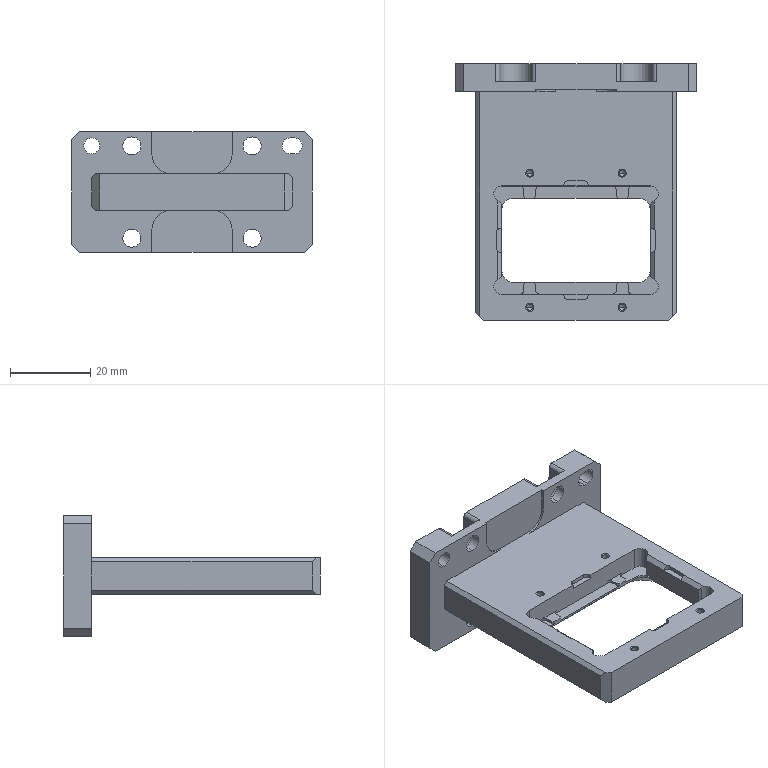NC program | NX | posted with a generic post | part box 60 x 64 x 30 mm
Lines 32 to 1126 of 12381:
(ZLEVEL_PROFILE , TOOL : D10)
N62 T10 M6
N64 G54
N66 G17 G0 G90 X-37.1 Y-22.891 B0. C0. S9500 M3
N68 G43 Z30. H10
N70 Z1.
N72 G94 G1 Y-18.973 Z0.795 F1000.
N74 X-37.107 Y-18.79 Z0.785
N76 X-37.1 Y-18.607 Z0.775
N78 Y-11.405 Z0.398
N80 X-37.107 Y-11.216 Z0.388
N82 X-37.1 Y-11. Z0.377
N84 Y0. Z-0.2
N86 Y11.027 F3000.
N88 G2 X-37.1 Y11.406 R5.116
N90 G1 Y18.608
N92 G2 X-37.1 Y19. R5.101
N94 G1 Y30.
N96 G2 X-32. Y35.1 R5.1
N98 G1 X-25.
N100 G2 X-19.901 Y30.1 R5.1
N102 G1 X30.
N104 G2 X33.606 Y28.606 R5.1
N106 G1 X35.606 Y26.606
N108 G2 X37.1 Y23. R5.1
N110 G1 Y-23.
N112 G2 X35.606 Y-26.606 R5.1
N114 G1 X33.606 Y-28.606
N116 G2 X30. Y-30.1 R5.1
N118 G1 X-19.901
N120 G2 X-25. Y-35.1 R5.1
N122 G1 X-32.
N124 G2 X-37.1 Y-30. R5.1
N126 G1 Y-18.973
N128 G2 X-37.1 Y-18.607 R5.115
N130 G1 Y-11.405
N132 G2 X-37.1 Y-11. R5.101
N134 G1 Y0.
N136 Y10.676 Z-0.386
N138 Y11.439 Z-0.399
N140 Y18.608
N142 G2 X-37.1 Y19. R5.101
N144 G1 Y30.
N146 G2 X-32. Y35.1 R5.1
N148 G1 X-25.
N150 G2 X-19.901 Y30.1 R5.1
N152 G1 X30.
N154 G2 X33.606 Y28.606 R5.1
N156 G1 X35.606 Y26.606
N158 G2 X37.1 Y23. R5.1
N160 G1 Y-23.
N162 G2 X35.606 Y-26.606 R5.1
N164 G1 X33.606 Y-28.606
N166 G2 X30. Y-30.1 R5.1
N168 G1 X-19.901
N170 G2 X-25. Y-35.1 R5.1
N172 G1 X-32.
N174 G2 X-37.1 Y-30. R5.1
N176 G1 Y-18.973
N178 G2 X-37.1 Y-18.607 R5.115
N180 G1 Y-11.405
N182 G2 X-37.1 Y-11. R5.101
N184 G1 Y0.
N186 Y10.676 Z-0.586
N188 Y11.439 Z-0.599
N190 Y18.608
N192 G2 X-37.1 Y19. R5.101
N194 G1 Y30.
N196 G2 X-32. Y35.1 R5.1
N198 G1 X-25.
N200 G2 X-19.901 Y30.1 R5.1
N202 G1 X30.
N204 G2 X33.606 Y28.606 R5.1
N206 G1 X35.606 Y26.606
N208 G2 X37.1 Y23. R5.1
N210 G1 Y-23.
N212 G2 X35.606 Y-26.606 R5.1
N214 G1 X33.606 Y-28.606
N216 G2 X30. Y-30.1 R5.1
N218 G1 X-19.901
N220 G2 X-25. Y-35.1 R5.1
N222 G1 X-32.
N224 G2 X-37.1 Y-30. R5.1
N226 G1 Y-18.973
N228 G2 X-37.1 Y-18.607 R5.115
N230 G1 Y-11.405
N232 G2 X-37.1 Y-11. R5.101
N234 G1 Y0.
N236 Y10.676 Z-0.785
N238 Y11.439 Z-0.799
N240 Y18.608
N242 G2 X-37.1 Y19. R5.101
N244 G1 Y30.
N246 G2 X-32. Y35.1 R5.1
N248 G1 X-25.
N250 G2 X-19.901 Y30.1 R5.1
N252 G1 X30.
N254 G2 X33.606 Y28.606 R5.1
N256 G1 X35.606 Y26.606
N258 G2 X37.1 Y23. R5.1
N260 G1 Y-23.
N262 G2 X35.606 Y-26.606 R5.1
N264 G1 X33.606 Y-28.606
N266 G2 X30. Y-30.1 R5.1
N268 G1 X-19.901
N270 G2 X-25. Y-35.1 R5.1
N272 G1 X-32.
N274 G2 X-37.1 Y-30. R5.1
N276 G1 Y-18.973
N278 G2 X-37.1 Y-18.607 R5.115
N280 G1 Y-11.405
N282 G2 X-37.1 Y-11. R5.101
N284 G1 Y0.
N286 Y10.676 Z-0.985
N288 Y11.439 Z-0.998
N290 Y18.608
N292 G2 X-37.1 Y19. R5.101
N294 G1 Y30.
N296 G2 X-32. Y35.1 R5.1
N298 G1 X-25.
N300 G2 X-19.901 Y30.1 R5.1
N302 G1 X30.
N304 G2 X33.606 Y28.606 R5.1
N306 G1 X35.606 Y26.606
N308 G2 X37.1 Y23. R5.1
N310 G1 Y-23.
N312 G2 X35.606 Y-26.606 R5.1
N314 G1 X33.606 Y-28.606
N316 G2 X30. Y-30.1 R5.1
N318 G1 X-19.901
N320 G2 X-25. Y-35.1 R5.1
N322 G1 X-32.
N324 G2 X-37.1 Y-30. R5.1
N326 G1 Y-18.973
N328 G2 X-37.1 Y-18.607 R5.115
N330 G1 Y-11.405
N332 G2 X-37.1 Y-11. R5.101
N334 G1 Y0.
N336 Y10.676 Z-1.185
N338 Y11.439 Z-1.198
N340 Y18.608
N342 G2 X-37.1 Y19. R5.101
N344 G1 Y30.
N346 G2 X-32. Y35.1 R5.1
N348 G1 X-25.
N350 G2 X-19.901 Y30.1 R5.1
N352 G1 X30.
N354 G2 X33.606 Y28.606 R5.1
N356 G1 X35.606 Y26.606
N358 G2 X37.1 Y23. R5.1
N360 G1 Y-23.
N362 G2 X35.606 Y-26.606 R5.1
N364 G1 X33.606 Y-28.606
N366 G2 X30. Y-30.1 R5.1
N368 G1 X-19.901
N370 G2 X-25. Y-35.1 R5.1
N372 G1 X-32.
N374 G2 X-37.1 Y-30. R5.1
N376 G1 Y-18.973
N378 G2 X-37.1 Y-18.607 R5.115
N380 G1 Y-11.405
N382 G2 X-37.1 Y-11. R5.101
N384 G1 Y0.
N386 Y10.676 Z-1.384
N388 Y11.439 Z-1.398
N390 Y18.608
N392 G2 X-37.1 Y19. R5.101
N394 G1 Y30.
N396 G2 X-32. Y35.1 R5.1
N398 G1 X-25.
N400 G2 X-19.901 Y30.1 R5.1
N402 G1 X30.
N404 G2 X33.606 Y28.606 R5.1
N406 G1 X35.606 Y26.606
N408 G2 X37.1 Y23. R5.1
N410 G1 Y-23.
N412 G2 X35.606 Y-26.606 R5.1
N414 G1 X33.606 Y-28.606
N416 G2 X30. Y-30.1 R5.1
N418 G1 X-19.901
N420 G2 X-25. Y-35.1 R5.1
N422 G1 X-32.
N424 G2 X-37.1 Y-30. R5.1
N426 G1 Y-18.973
N428 G2 X-37.1 Y-18.607 R5.115
N430 G1 Y-11.405
N432 G2 X-37.1 Y-11. R5.101
N434 G1 Y0.
N436 Y10.676 Z-1.584
N438 Y11.439 Z-1.597
N440 Y18.608
N442 G2 X-37.1 Y19. R5.101
N444 G1 Y30.
N446 G2 X-32. Y35.1 R5.1
N448 G1 X-25.
N450 G2 X-19.901 Y30.1 R5.1
N452 G1 X30.
N454 G2 X33.606 Y28.606 R5.1
N456 G1 X35.606 Y26.606
N458 G2 X37.1 Y23. R5.1
N460 G1 Y-23.
N462 G2 X35.606 Y-26.606 R5.1
N464 G1 X33.606 Y-28.606
N466 G2 X30. Y-30.1 R5.1
N468 G1 X-19.901
N470 G2 X-25. Y-35.1 R5.1
N472 G1 X-32.
N474 G2 X-37.1 Y-30. R5.1
N476 G1 Y-18.973
N478 G2 X-37.1 Y-18.607 R5.115
N480 G1 Y-11.405
N482 G2 X-37.1 Y-11. R5.101
N484 G1 Y0.
N486 Y10.676 Z-1.784
N488 Y11.439 Z-1.797
N490 Y18.608
N492 G2 X-37.1 Y19. R5.101
N494 G1 Y30.
N496 G2 X-32. Y35.1 R5.1
N498 G1 X-25.
N500 G2 X-19.901 Y30.1 R5.1
N502 G1 X30.
N504 G2 X33.606 Y28.606 R5.1
N506 G1 X35.606 Y26.606
N508 G2 X37.1 Y23. R5.1
N510 G1 Y-23.
N512 G2 X35.606 Y-26.606 R5.1
N514 G1 X33.606 Y-28.606
N516 G2 X30. Y-30.1 R5.1
N518 G1 X-19.901
N520 G2 X-25. Y-35.1 R5.1
N522 G1 X-32.
N524 G2 X-37.1 Y-30. R5.1
N526 G1 Y-18.973
N528 G2 X-37.1 Y-18.607 R5.115
N530 G1 Y-11.405
N532 G2 X-37.1 Y-11. R5.101
N534 G1 Y0.
N536 Y10.676 Z-1.983
N538 Y11.439 Z-1.997
N540 Y18.608
N542 G2 X-37.1 Y19. R5.101
N544 G1 Y30.
N546 G2 X-32. Y35.1 R5.1
N548 G1 X-25.
N550 G2 X-19.901 Y30.1 R5.1
N552 G1 X30.
N554 G2 X33.606 Y28.606 R5.1
N556 G1 X35.606 Y26.606
N558 G2 X37.1 Y23. R5.1
N560 G1 Y-23.
N562 G2 X35.606 Y-26.606 R5.1
N564 G1 X33.606 Y-28.606
N566 G2 X30. Y-30.1 R5.1
N568 G1 X-19.901
N570 G2 X-25. Y-35.1 R5.1
N572 G1 X-32.
N574 G2 X-37.1 Y-30. R5.1
N576 G1 Y-18.973
N578 G2 X-37.1 Y-18.607 R5.115
N580 G1 Y-11.405
N582 G2 X-37.1 Y-11. R5.101
N584 G1 Y0.
N586 Y10.676 Z-2.183
N588 Y11.439 Z-2.196
N590 Y18.608
N592 G2 X-37.1 Y19. R5.101
N594 G1 Y30.
N596 G2 X-32. Y35.1 R5.1
N598 G1 X-25.
N600 G2 X-19.901 Y30.1 R5.1
N602 G1 X30.
N604 G2 X33.606 Y28.606 R5.1
N606 G1 X35.606 Y26.606
N608 G2 X37.1 Y23. R5.1
N610 G1 Y-23.
N612 G2 X35.606 Y-26.606 R5.1
N614 G1 X33.606 Y-28.606
N616 G2 X30. Y-30.1 R5.1
N618 G1 X-19.901
N620 G2 X-25. Y-35.1 R5.1
N622 G1 X-32.
N624 G2 X-37.1 Y-30. R5.1
N626 G1 Y-18.973
N628 G2 X-37.1 Y-18.607 R5.115
N630 G1 Y-11.405
N632 G2 X-37.1 Y-11. R5.101
N634 G1 Y0.
N636 Y10.676 Z-2.383
N638 Y11.439 Z-2.396
N640 Y18.608
N642 G2 X-37.1 Y19. R5.101
N644 G1 Y30.
N646 G2 X-32. Y35.1 R5.1
N648 G1 X-25.
N650 G2 X-19.901 Y30.1 R5.1
N652 G1 X30.
N654 G2 X33.606 Y28.606 R5.1
N656 G1 X35.606 Y26.606
N658 G2 X37.1 Y23. R5.1
N660 G1 Y-23.
N662 G2 X35.606 Y-26.606 R5.1
N664 G1 X33.606 Y-28.606
N666 G2 X30. Y-30.1 R5.1
N668 G1 X-19.901
N670 G2 X-25. Y-35.1 R5.1
N672 G1 X-32.
N674 G2 X-37.1 Y-30. R5.1
N676 G1 Y-18.973
N678 G2 X-37.1 Y-18.607 R5.115
N680 G1 Y-11.405
N682 G2 X-37.1 Y-11. R5.101
N684 G1 Y0.
N686 Y10.676 Z-2.582
N688 Y11.439 Z-2.596
N690 Y18.608
N692 G2 X-37.1 Y19. R5.101
N694 G1 Y30.
N696 G2 X-32. Y35.1 R5.1
N698 G1 X-25.
N700 G2 X-19.901 Y30.1 R5.1
N702 G1 X30.
N704 G2 X33.606 Y28.606 R5.1
N706 G1 X35.606 Y26.606
N708 G2 X37.1 Y23. R5.1
N710 G1 Y-23.
N712 G2 X35.606 Y-26.606 R5.1
N714 G1 X33.606 Y-28.606
N716 G2 X30. Y-30.1 R5.1
N718 G1 X-19.901
N720 G2 X-25. Y-35.1 R5.1
N722 G1 X-32.
N724 G2 X-37.1 Y-30. R5.1
N726 G1 Y-18.973
N728 G2 X-37.1 Y-18.607 R5.115
N730 G1 Y-11.405
N732 G2 X-37.1 Y-11. R5.101
N734 G1 Y0.
N736 Y10.676 Z-2.782
N738 Y11.439 Z-2.795
N740 Y18.608
N742 G2 X-37.1 Y19. R5.101
N744 G1 Y30.
N746 G2 X-32. Y35.1 R5.1
N748 G1 X-25.
N750 G2 X-19.901 Y30.1 R5.1
N752 G1 X30.
N754 G2 X33.606 Y28.606 R5.1
N756 G1 X35.606 Y26.606
N758 G2 X37.1 Y23. R5.1
N760 G1 Y-23.
N762 G2 X35.606 Y-26.606 R5.1
N764 G1 X33.606 Y-28.606
N766 G2 X30. Y-30.1 R5.1
N768 G1 X-19.901
N770 G2 X-25. Y-35.1 R5.1
N772 G1 X-32.
N774 G2 X-37.1 Y-30. R5.1
N776 G1 Y-18.973
N778 G2 X-37.1 Y-18.607 R5.115
N780 G1 Y-11.405
N782 G2 X-37.1 Y-11. R5.101
N784 G1 Y0.
N786 Y10.676 Z-2.982
N788 Y11.439 Z-2.995
N790 Y18.608
N792 G2 X-37.1 Y19. R5.101
N794 G1 Y30.
N796 G2 X-32. Y35.1 R5.1
N798 G1 X-25.
N800 G2 X-19.901 Y30.1 R5.1
N802 G1 X30.
N804 G2 X33.606 Y28.606 R5.1
N806 G1 X35.606 Y26.606
N808 G2 X37.1 Y23. R5.1
N810 G1 Y-23.
N812 G2 X35.606 Y-26.606 R5.1
N814 G1 X33.606 Y-28.606
N816 G2 X30. Y-30.1 R5.1
N818 G1 X-19.901
N820 G2 X-25. Y-35.1 R5.1
N822 G1 X-32.
N824 G2 X-37.1 Y-30. R5.1
N826 G1 Y-18.973
N828 G2 X-37.1 Y-18.607 R5.115
N830 G1 Y-11.405
N832 G2 X-37.1 Y-11. R5.101
N834 G1 Y0.
N836 Y10.676 Z-3.181
N838 Y11.439 Z-3.195
N840 Y18.608
N842 G2 X-37.1 Y19. R5.101
N844 G1 Y30.
N846 G2 X-32. Y35.1 R5.1
N848 G1 X-25.
N850 G2 X-19.901 Y30.1 R5.1
N852 G1 X30.
N854 G2 X33.606 Y28.606 R5.1
N856 G1 X35.606 Y26.606
N858 G2 X37.1 Y23. R5.1
N860 G1 Y-23.
N862 G2 X35.606 Y-26.606 R5.1
N864 G1 X33.606 Y-28.606
N866 G2 X30. Y-30.1 R5.1
N868 G1 X-19.901
N870 G2 X-25. Y-35.1 R5.1
N872 G1 X-32.
N874 G2 X-37.1 Y-30. R5.1
N876 G1 Y-18.973
N878 G2 X-37.1 Y-18.607 R5.115
N880 G1 Y-11.405
N882 G2 X-37.1 Y-11. R5.101
N884 G1 Y0.
N886 Y10.676 Z-3.381
N888 Y11.439 Z-3.394
N890 Y18.608
N892 G2 X-37.1 Y19. R5.101
N894 G1 Y30.
N896 G2 X-32. Y35.1 R5.1
N898 G1 X-25.
N900 G2 X-19.901 Y30.1 R5.1
N902 G1 X30.
N904 G2 X33.606 Y28.606 R5.1
N906 G1 X35.606 Y26.606
N908 G2 X37.1 Y23. R5.1
N910 G1 Y-23.
N912 G2 X35.606 Y-26.606 R5.1
N914 G1 X33.606 Y-28.606
N916 G2 X30. Y-30.1 R5.1
N918 G1 X-19.901
N920 G2 X-25. Y-35.1 R5.1
N922 G1 X-32.
N924 G2 X-37.1 Y-30. R5.1
N926 G1 Y-18.973
N928 G2 X-37.1 Y-18.607 R5.115
N930 G1 Y-11.405
N932 G2 X-37.1 Y-11. R5.101
N934 G1 Y0.
N936 Y10.676 Z-3.581
N938 Y11.439 Z-3.594
N940 Y18.608
N942 G2 X-37.1 Y19. R5.101
N944 G1 Y30.
N946 G2 X-32. Y35.1 R5.1
N948 G1 X-25.
N950 G2 X-19.901 Y30.1 R5.1
N952 G1 X30.
N954 G2 X33.606 Y28.606 R5.1
N956 G1 X35.606 Y26.606
N958 G2 X37.1 Y23. R5.1
N960 G1 Y-23.
N962 G2 X35.606 Y-26.606 R5.1
N964 G1 X33.606 Y-28.606
N966 G2 X30. Y-30.1 R5.1
N968 G1 X-19.901
N970 G2 X-25. Y-35.1 R5.1
N972 G1 X-32.
N974 G2 X-37.1 Y-30. R5.1
N976 G1 Y-18.973
N978 G2 X-37.1 Y-18.607 R5.115
N980 G1 Y-11.405
N982 G2 X-37.1 Y-11. R5.101
N984 G1 Y0.
N986 Y10.676 Z-3.78
N988 Y11.439 Z-3.794
N990 Y18.608
N992 G2 X-37.1 Y19. R5.101
N994 G1 Y30.
N996 G2 X-32. Y35.1 R5.1
N998 G1 X-25.
N1000 G2 X-19.901 Y30.1 R5.1
N1002 G1 X30.
N1004 G2 X33.606 Y28.606 R5.1
N1006 G1 X35.606 Y26.606
N1008 G2 X37.1 Y23. R5.1
N1010 G1 Y-23.
N1012 G2 X35.606 Y-26.606 R5.1
N1014 G1 X33.606 Y-28.606
N1016 G2 X30. Y-30.1 R5.1
N1018 G1 X-19.901
N1020 G2 X-25. Y-35.1 R5.1
N1022 G1 X-32.
N1024 G2 X-37.1 Y-30. R5.1
N1026 G1 Y-18.973
N1028 G2 X-37.1 Y-18.607 R5.115
N1030 G1 Y-11.405
N1032 G2 X-37.1 Y-11. R5.101
N1034 G1 Y0.
N1036 Y10.676 Z-3.98
N1038 Y11.439 Z-3.993
N1040 Y18.608
N1042 G2 X-37.1 Y19. R5.101
N1044 G1 Y30.
N1046 G2 X-32. Y35.1 R5.1
N1048 G1 X-25.
N1050 G2 X-19.901 Y30.1 R5.1
N1052 G1 X30.
N1054 G2 X33.606 Y28.606 R5.1
N1056 G1 X35.606 Y26.606
N1058 G2 X37.1 Y23. R5.1
N1060 G1 Y-23.
N1062 G2 X35.606 Y-26.606 R5.1
N1064 G1 X33.606 Y-28.606
N1066 G2 X30. Y-30.1 R5.1
N1068 G1 X-19.901
N1070 G2 X-25. Y-35.1 R5.1
N1072 G1 X-32.
N1074 G2 X-37.1 Y-30. R5.1
N1076 G1 Y-18.973
N1078 G2 X-37.1 Y-18.607 R5.115
N1080 G1 Y-11.405
N1082 G2 X-37.1 Y-11. R5.101
N1084 G1 Y0.
N1086 Y10.676 Z-4.18
N1088 Y11.439 Z-4.193
N1090 Y18.608
N1092 G2 X-37.1 Y19. R5.101
N1094 G1 Y30.
N1096 G2 X-32. Y35.1 R5.1
N1098 G1 X-25.
N1100 G2 X-19.901 Y30.1 R5.1
N1102 G1 X30.
N1104 G2 X33.606 Y28.606 R5.1
N1106 G1 X35.606 Y26.606
N1108 G2 X37.1 Y23. R5.1
N1110 G1 Y-23.
N1112 G2 X35.606 Y-26.606 R5.1
N1114 G1 X33.606 Y-28.606
N1116 G2 X30. Y-30.1 R5.1
N1118 G1 X-19.901
N1120 G2 X-25. Y-35.1 R5.1
N1122 G1 X-32.
N1124 G2 X-37.1 Y-30. R5.1
N1126 G1 Y-18.973
N1128 G2 X-37.1 Y-18.607 R5.115
N1130 G1 Y-11.405
N1132 G2 X-37.1 Y-11. R5.101
N1134 G1 Y0.
N1136 Y10.676 Z-4.379
N1138 Y11.439 Z-4.393
N1140 Y18.608
N1142 G2 X-37.1 Y19. R5.101
N1144 G1 Y30.
N1146 G2 X-32. Y35.1 R5.1
N1148 G1 X-25.
N1150 G2 X-19.901 Y30.1 R5.1
N1152 G1 X30.
N1154 G2 X33.606 Y28.606 R5.1
N1156 G1 X35.606 Y26.606
N1158 G2 X37.1 Y23. R5.1
N1160 G1 Y-23.
N1162 G2 X35.606 Y-26.606 R5.1
N1164 G1 X33.606 Y-28.606
N1166 G2 X30. Y-30.1 R5.1
N1168 G1 X-19.901
N1170 G2 X-25. Y-35.1 R5.1
N1172 G1 X-32.
N1174 G2 X-37.1 Y-30. R5.1
N1176 G1 Y-18.973
N1178 G2 X-37.1 Y-18.607 R5.115
N1180 G1 Y-11.405
N1182 G2 X-37.1 Y-11. R5.101
N1184 G1 Y0.
N1186 Y10.676 Z-4.579
N1188 Y11.439 Z-4.592
N1190 Y18.608
N1192 G2 X-37.1 Y19. R5.101
N1194 G1 Y30.
N1196 G2 X-32. Y35.1 R5.1
N1198 G1 X-25.
N1200 G2 X-19.901 Y30.1 R5.1
N1202 G1 X30.
N1204 G2 X33.606 Y28.606 R5.1
N1206 G1 X35.606 Y26.606
N1208 G2 X37.1 Y23. R5.1
N1210 G1 Y-23.
N1212 G2 X35.606 Y-26.606 R5.1
N1214 G1 X33.606 Y-28.606
N1216 G2 X30. Y-30.1 R5.1
N1218 G1 X-19.901
N1220 G2 X-25. Y-35.1 R5.1
N1222 G1 X-32.
N1224 G2 X-37.1 Y-30. R5.1
N1226 G1 Y-18.973
N1228 G2 X-37.1 Y-18.607 R5.115
N1230 G1 Y-11.405
N1232 G2 X-37.1 Y-11. R5.101
N1234 G1 Y0.
N1236 Y10.676 Z-4.779
N1238 Y11.439 Z-4.792
N1240 Y18.608
N1242 G2 X-37.1 Y19. R5.101
N1244 G1 Y30.
N1246 G2 X-32. Y35.1 R5.1
N1248 G1 X-25.
N1250 G2 X-19.901 Y30.1 R5.1
N1252 G1 X30.
N1254 G2 X33.606 Y28.606 R5.1
N1256 G1 X35.606 Y26.606
N1258 G2 X37.1 Y23. R5.1
N1260 G1 Y-23.
N1262 G2 X35.606 Y-26.606 R5.1
N1264 G1 X33.606 Y-28.606
N1266 G2 X30. Y-30.1 R5.1
N1268 G1 X-19.901
N1270 G2 X-25. Y-35.1 R5.1
N1272 G1 X-32.
N1274 G2 X-37.1 Y-30. R5.1
N1276 G1 Y-18.973
N1278 G2 X-37.1 Y-18.607 R5.115
N1280 G1 Y-11.405
N1282 G2 X-37.1 Y-11. R5.101
N1284 G1 Y0.
N1286 Y10.676 Z-4.978
N1288 Y11.439 Z-4.992
N1290 Y18.608
N1292 G2 X-37.1 Y19. R5.101
N1294 G1 Y30.
N1296 G2 X-32. Y35.1 R5.1
N1298 G1 X-25.
N1300 G2 X-19.901 Y30.1 R5.1
N1302 G1 X30.
N1304 G2 X33.606 Y28.606 R5.1
N1306 G1 X35.606 Y26.606
N1308 G2 X37.1 Y23. R5.1
N1310 G1 Y-23.
N1312 G2 X35.606 Y-26.606 R5.1
N1314 G1 X33.606 Y-28.606
N1316 G2 X30. Y-30.1 R5.1
N1318 G1 X-19.901
N1320 G2 X-25. Y-35.1 R5.1
N1322 G1 X-32.
N1324 G2 X-37.1 Y-30. R5.1
N1326 G1 Y-18.973
N1328 G2 X-37.1 Y-18.607 R5.115
N1330 G1 Y-11.405
N1332 G2 X-37.1 Y-11. R5.101
N1334 G1 Y0.
N1336 Y10.676 Z-5.178
N1338 Y11.439 Z-5.191
N1340 Y18.608
N1342 G2 X-37.1 Y19. R5.101
N1344 G1 Y30.
N1346 G2 X-32. Y35.1 R5.1
N1348 G1 X-25.
N1350 G2 X-19.901 Y30.1 R5.1
N1352 G1 X30.
N1354 G2 X33.606 Y28.606 R5.1
N1356 G1 X35.606 Y26.606
N1358 G2 X37.1 Y23. R5.1
N1360 G1 Y-23.
N1362 G2 X35.606 Y-26.606 R5.1
N1364 G1 X33.606 Y-28.606
N1366 G2 X30. Y-30.1 R5.1
N1368 G1 X-19.901
N1370 G2 X-25. Y-35.1 R5.1
N1372 G1 X-32.
N1374 G2 X-37.1 Y-30. R5.1
N1376 G1 Y-18.973
N1378 G2 X-37.1 Y-18.607 R5.115
N1380 G1 Y-11.405
N1382 G2 X-37.1 Y-11. R5.101
N1384 G1 Y0.
N1386 Y10.676 Z-5.378
N1388 Y11.439 Z-5.391
N1390 Y18.608
N1392 G2 X-37.1 Y19. R5.101
N1394 G1 Y30.
N1396 G2 X-32. Y35.1 R5.1
N1398 G1 X-25.
N1400 G2 X-19.901 Y30.1 R5.1
N1402 G1 X30.
N1404 G2 X33.606 Y28.606 R5.1
N1406 G1 X35.606 Y26.606
N1408 G2 X37.1 Y23. R5.1
N1410 G1 Y-23.
N1412 G2 X35.606 Y-26.606 R5.1
N1414 G1 X33.606 Y-28.606
N1416 G2 X30. Y-30.1 R5.1
N1418 G1 X-19.901
N1420 G2 X-25. Y-35.1 R5.1
N1422 G1 X-32.
N1424 G2 X-37.1 Y-30. R5.1
N1426 G1 Y-18.973
N1428 G2 X-37.1 Y-18.607 R5.115
N1430 G1 Y-11.405
N1432 G2 X-37.1 Y-11. R5.101
N1434 G1 Y0.
N1436 Y10.676 Z-5.577
N1438 Y11.439 Z-5.591
N1440 Y18.608
N1442 G2 X-37.1 Y19. R5.101
N1444 G1 Y30.
N1446 G2 X-32. Y35.1 R5.1
N1448 G1 X-25.
N1450 G2 X-19.901 Y30.1 R5.1
N1452 G1 X30.
N1454 G2 X33.606 Y28.606 R5.1
N1456 G1 X35.606 Y26.606
N1458 G2 X37.1 Y23. R5.1
N1460 G1 Y-23.
N1462 G2 X35.606 Y-26.606 R5.1
N1464 G1 X33.606 Y-28.606
N1466 G2 X30. Y-30.1 R5.1
N1468 G1 X-19.901
N1470 G2 X-25. Y-35.1 R5.1
N1472 G1 X-32.
N1474 G2 X-37.1 Y-30. R5.1
N1476 G1 Y-18.973
N1478 G2 X-37.1 Y-18.607 R5.115
N1480 G1 Y-11.405
N1482 G2 X-37.1 Y-11. R5.101
N1484 G1 Y0.
N1486 Y10.676 Z-5.777
N1488 Y11.439 Z-5.79
N1490 Y18.608
N1492 G2 X-37.1 Y19. R5.101
N1494 G1 Y30.
N1496 G2 X-32. Y35.1 R5.1
N1498 G1 X-25.
N1500 G2 X-19.901 Y30.1 R5.1
N1502 G1 X30.
N1504 G2 X33.606 Y28.606 R5.1
N1506 G1 X35.606 Y26.606
N1508 G2 X37.1 Y23. R5.1
N1510 G1 Y-23.
N1512 G2 X35.606 Y-26.606 R5.1
N1514 G1 X33.606 Y-28.606
N1516 G2 X30. Y-30.1 R5.1
N1518 G1 X-19.901
N1520 G2 X-25. Y-35.1 R5.1
N1522 G1 X-32.
N1524 G2 X-37.1 Y-30. R5.1
N1526 G1 Y-18.973
N1528 G2 X-37.1 Y-18.607 R5.115
N1530 G1 Y-11.405
N1532 G2 X-37.1 Y-11. R5.101
N1534 G1 Y0.
N1536 Y10.676 Z-5.977
N1538 Y11.439 Z-5.99
N1540 Y18.608
N1542 G2 X-37.1 Y19. R5.101
N1544 G1 Y30.
N1546 G2 X-32. Y35.1 R5.1
N1548 G1 X-25.
N1550 G2 X-19.901 Y30.1 R5.1
N1552 G1 X30.
N1554 G2 X33.606 Y28.606 R5.1
N1556 G1 X35.606 Y26.606
N1558 G2 X37.1 Y23. R5.1
N1560 G1 Y-23.
N1562 G2 X35.606 Y-26.606 R5.1
N1564 G1 X33.606 Y-28.606
N1566 G2 X30. Y-30.1 R5.1
N1568 G1 X-19.901
N1570 G2 X-25. Y-35.1 R5.1
N1572 G1 X-32.
N1574 G2 X-37.1 Y-30. R5.1
N1576 G1 Y-18.973
N1578 G2 X-37.1 Y-18.607 R5.115
N1580 G1 Y-11.405
N1582 G2 X-37.1 Y-11. R5.101
N1584 G1 Y0.
N1586 Y10.676 Z-6.176
N1588 Y11.439 Z-6.19
N1590 Y18.608
N1592 G2 X-37.1 Y19. R5.101
N1594 G1 Y30.
N1596 G2 X-32. Y35.1 R5.1
N1598 G1 X-25.
N1600 G2 X-19.901 Y30.1 R5.1
N1602 G1 X30.
N1604 G2 X33.606 Y28.606 R5.1
N1606 G1 X35.606 Y26.606
N1608 G2 X37.1 Y23. R5.1
N1610 G1 Y-23.
N1612 G2 X35.606 Y-26.606 R5.1
N1614 G1 X33.606 Y-28.606
N1616 G2 X30. Y-30.1 R5.1
N1618 G1 X-19.901
N1620 G2 X-25. Y-35.1 R5.1
N1622 G1 X-32.
N1624 G2 X-37.1 Y-30. R5.1
N1626 G1 Y-18.973
N1628 G2 X-37.1 Y-18.607 R5.115
N1630 G1 Y-11.405
N1632 G2 X-37.1 Y-11. R5.101
N1634 G1 Y0.
N1636 Y10.676 Z-6.376
N1638 Y11.439 Z-6.389
N1640 Y18.608
N1642 G2 X-37.1 Y19. R5.101
N1644 G1 Y30.
N1646 G2 X-32. Y35.1 R5.1
N1648 G1 X-25.
N1650 G2 X-19.901 Y30.1 R5.1
N1652 G1 X30.
N1654 G2 X33.606 Y28.606 R5.1
N1656 G1 X35.606 Y26.606
N1658 G2 X37.1 Y23. R5.1
N1660 G1 Y-23.
N1662 G2 X35.606 Y-26.606 R5.1
N1664 G1 X33.606 Y-28.606
N1666 G2 X30. Y-30.1 R5.1
N1668 G1 X-19.901
N1670 G2 X-25. Y-35.1 R5.1
N1672 G1 X-32.
N1674 G2 X-37.1 Y-30. R5.1
N1676 G1 Y-18.973
N1678 G2 X-37.1 Y-18.607 R5.115
N1680 G1 Y-11.405
N1682 G2 X-37.1 Y-11. R5.101
N1684 G1 Y0.
N1686 Y10.676 Z-6.576
N1688 Y11.439 Z-6.589
N1690 Y18.608
N1692 G2 X-37.1 Y19. R5.101
N1694 G1 Y30.
N1696 G2 X-32. Y35.1 R5.1
N1698 G1 X-25.
N1700 G2 X-19.901 Y30.1 R5.1
N1702 G1 X30.
N1704 G2 X33.606 Y28.606 R5.1
N1706 G1 X35.606 Y26.606
N1708 G2 X37.1 Y23. R5.1
N1710 G1 Y-23.
N1712 G2 X35.606 Y-26.606 R5.1
N1714 G1 X33.606 Y-28.606
N1716 G2 X30. Y-30.1 R5.1
N1718 G1 X-19.901
N1720 G2 X-25. Y-35.1 R5.1
N1722 G1 X-32.
N1724 G2 X-37.1 Y-30. R5.1
N1726 G1 Y-18.973
N1728 G2 X-37.1 Y-18.607 R5.115
N1730 G1 Y-11.405
N1732 G2 X-37.1 Y-11. R5.101
N1734 G1 Y0.
N1736 Y10.676 Z-6.775
N1738 Y11.439 Z-6.789
N1740 Y18.608
N1742 G2 X-37.1 Y19. R5.101
N1744 G1 Y30.
N1746 G2 X-32. Y35.1 R5.1
N1748 G1 X-25.
N1750 G2 X-19.901 Y30.1 R5.1
N1752 G1 X30.
N1754 G2 X33.606 Y28.606 R5.1
N1756 G1 X35.606 Y26.606
N1758 G2 X37.1 Y23. R5.1
N1760 G1 Y-23.
N1762 G2 X35.606 Y-26.606 R5.1
N1764 G1 X33.606 Y-28.606
N1766 G2 X30. Y-30.1 R5.1
N1768 G1 X-19.901
N1770 G2 X-25. Y-35.1 R5.1
N1772 G1 X-32.
N1774 G2 X-37.1 Y-30. R5.1
N1776 G1 Y-18.973
N1778 G2 X-37.1 Y-18.607 R5.115
N1780 G1 Y-11.405
N1782 G2 X-37.1 Y-11. R5.101
N1784 G1 Y0.
N1786 Y10.676 Z-6.975
N1788 Y11.439 Z-6.988
N1790 Y18.608
N1792 G2 X-37.1 Y19. R5.101
N1794 G1 Y30.
N1796 G2 X-32. Y35.1 R5.1
N1798 G1 X-25.
N1800 G2 X-19.901 Y30.1 R5.1
N1802 G1 X30.
N1804 G2 X33.606 Y28.606 R5.1
N1806 G1 X35.606 Y26.606
N1808 G2 X37.1 Y23. R5.1
N1810 G1 Y-23.
N1812 G2 X35.606 Y-26.606 R5.1
N1814 G1 X33.606 Y-28.606
N1816 G2 X30. Y-30.1 R5.1
N1818 G1 X-19.901
N1820 G2 X-25. Y-35.1 R5.1
N1822 G1 X-32.
N1824 G2 X-37.1 Y-30. R5.1
N1826 G1 Y-18.973
N1828 G2 X-37.1 Y-18.607 R5.115
N1830 G1 Y-11.405
N1832 G2 X-37.1 Y-11. R5.101
N1834 G1 Y0.
N1836 Y10.676 Z-7.175
N1838 Y11.439 Z-7.188
N1840 Y18.608
N1842 G2 X-37.1 Y19. R5.101
N1844 G1 Y30.
N1846 G2 X-32. Y35.1 R5.1
N1848 G1 X-25.
N1850 G2 X-19.901 Y30.1 R5.1
N1852 G1 X30.
N1854 G2 X33.606 Y28.606 R5.1
N1856 G1 X35.606 Y26.606
N1858 G2 X37.1 Y23. R5.1
N1860 G1 Y-23.
N1862 G2 X35.606 Y-26.606 R5.1
N1864 G1 X33.606 Y-28.606
N1866 G2 X30. Y-30.1 R5.1
N1868 G1 X-19.901
N1870 G2 X-25. Y-35.1 R5.1
N1872 G1 X-32.
N1874 G2 X-37.1 Y-30. R5.1
N1876 G1 Y-18.973
N1878 G2 X-37.1 Y-18.607 R5.115
N1880 G1 Y-11.405
N1882 G2 X-37.1 Y-11. R5.101
N1884 G1 Y0.
N1886 Y10.676 Z-7.374
N1888 Y11.439 Z-7.388
N1890 Y18.608
N1892 G2 X-37.1 Y19. R5.101
N1894 G1 Y30.
N1896 G2 X-32. Y35.1 R5.1
N1898 G1 X-25.
N1900 G2 X-19.901 Y30.1 R5.1
N1902 G1 X30.
N1904 G2 X33.606 Y28.606 R5.1
N1906 G1 X35.606 Y26.606
N1908 G2 X37.1 Y23. R5.1
N1910 G1 Y-23.
N1912 G2 X35.606 Y-26.606 R5.1
N1914 G1 X33.606 Y-28.606
N1916 G2 X30. Y-30.1 R5.1
N1918 G1 X-19.901
N1920 G2 X-25. Y-35.1 R5.1
N1922 G1 X-32.
N1924 G2 X-37.1 Y-30. R5.1
N1926 G1 Y-18.973
N1928 G2 X-37.1 Y-18.607 R5.115
N1930 G1 Y-11.405
N1932 G2 X-37.1 Y-11. R5.101
N1934 G1 Y0.
N1936 Y10.676 Z-7.574
N1938 Y11.439 Z-7.587
N1940 Y18.608
N1942 G2 X-37.1 Y19. R5.101
N1944 G1 Y30.
N1946 G2 X-32. Y35.1 R5.1
N1948 G1 X-25.
N1950 G2 X-19.901 Y30.1 R5.1
N1952 G1 X30.
N1954 G2 X33.606 Y28.606 R5.1
N1956 G1 X35.606 Y26.606
N1958 G2 X37.1 Y23. R5.1
N1960 G1 Y-23.
N1962 G2 X35.606 Y-26.606 R5.1
N1964 G1 X33.606 Y-28.606
N1966 G2 X30. Y-30.1 R5.1
N1968 G1 X-19.901
N1970 G2 X-25. Y-35.1 R5.1
N1972 G1 X-32.
N1974 G2 X-37.1 Y-30. R5.1
N1976 G1 Y-18.973
N1978 G2 X-37.1 Y-18.607 R5.115
N1980 G1 Y-11.405
N1982 G2 X-37.1 Y-11. R5.101
N1984 G1 Y0.
N1986 Y10.676 Z-7.774
N1988 Y11.439 Z-7.787
N1990 Y18.608
N1992 G2 X-37.1 Y19. R5.101
N1994 G1 Y30.
N1996 G2 X-32. Y35.1 R5.1
N1998 G1 X-25.
N2000 G2 X-19.901 Y30.1 R5.1
N2002 G1 X30.
N2004 G2 X33.606 Y28.606 R5.1
N2006 G1 X35.606 Y26.606
N2008 G2 X37.1 Y23. R5.1
N2010 G1 Y-23.
N2012 G2 X35.606 Y-26.606 R5.1
N2014 G1 X33.606 Y-28.606
N2016 G2 X30. Y-30.1 R5.1
N2018 G1 X-19.901
N2020 G2 X-25. Y-35.1 R5.1
N2022 G1 X-32.
N2024 G2 X-37.1 Y-30. R5.1
N2026 G1 Y-18.973
N2028 G2 X-37.1 Y-18.607 R5.115
N2030 G1 Y-11.405
N2032 G2 X-37.1 Y-11. R5.101
N2034 G1 Y0.
N2036 Y10.676 Z-7.973
N2038 Y11.439 Z-7.987
N2040 Y18.608
N2042 G2 X-37.1 Y19. R5.101
N2044 G1 Y30.
N2046 G2 X-32. Y35.1 R5.1
N2048 G1 X-25.
N2050 G2 X-19.901 Y30.1 R5.1
N2052 G1 X30.
N2054 G2 X33.606 Y28.606 R5.1
N2056 G1 X35.606 Y26.606
N2058 G2 X37.1 Y23. R5.1
N2060 G1 Y-23.
N2062 G2 X35.606 Y-26.606 R5.1
N2064 G1 X33.606 Y-28.606
N2066 G2 X30. Y-30.1 R5.1
N2068 G1 X-19.901
N2070 G2 X-25. Y-35.1 R5.1
N2072 G1 X-32.
N2074 G2 X-37.1 Y-30. R5.1
N2076 G1 Y-18.973
N2078 G2 X-37.1 Y-18.607 R5.115
N2080 G1 Y-11.405
N2082 G2 X-37.1 Y-11. R5.101
N2084 G1 Y0.
N2086 Y10.676 Z-8.173
N2088 Y11.439 Z-8.186
N2090 Y18.608
N2092 G2 X-37.1 Y19. R5.101
N2094 G1 Y30.
N2096 G2 X-32. Y35.1 R5.1
N2098 G1 X-25.
N2100 G2 X-19.901 Y30.1 R5.1
N2102 G1 X30.
N2104 G2 X33.606 Y28.606 R5.1
N2106 G1 X35.606 Y26.606
N2108 G2 X37.1 Y23. R5.1
N2110 G1 Y-23.
N2112 G2 X35.606 Y-26.606 R5.1
N2114 G1 X33.606 Y-28.606
N2116 G2 X30. Y-30.1 R5.1
N2118 G1 X-19.901
N2120 G2 X-25. Y-35.1 R5.1
N2122 G1 X-32.
N2124 G2 X-37.1 Y-30. R5.1
N2126 G1 Y-18.973
N2128 G2 X-37.1 Y-18.607 R5.115
N2130 G1 Y-11.405
N2132 G2 X-37.1 Y-11. R5.101
N2134 G1 Y0.
N2136 Y10.676 Z-8.373
N2138 Y11.439 Z-8.386
N2140 Y18.608
N2142 G2 X-37.1 Y19. R5.101
N2144 G1 Y30.
N2146 G2 X-32. Y35.1 R5.1
N2148 G1 X-25.
N2150 G2 X-19.901 Y30.1 R5.1
N2152 G1 X30.
N2154 G2 X33.606 Y28.606 R5.1
N2156 G1 X35.606 Y26.606
N2158 G2 X37.1 Y23. R5.1
N2160 G1 Y-23.
N2162 G2 X35.606 Y-26.606 R5.1
N2164 G1 X33.606 Y-28.606
N2166 G2 X30. Y-30.1 R5.1
N2168 G1 X-19.901
N2170 G2 X-25. Y-35.1 R5.1
N2172 G1 X-32.
N2174 G2 X-37.1 Y-30. R5.1
N2176 G1 Y-18.973
N2178 G2 X-37.1 Y-18.607 R5.115
N2180 G1 Y-11.405
N2182 G2 X-37.1 Y-11. R5.101
N2184 G1 Y0.
N2186 Y10.676 Z-8.572
N2188 Y11.439 Z-8.586
N2190 Y18.608
N2192 G2 X-37.1 Y19. R5.101
N2194 G1 Y30.
N2196 G2 X-32. Y35.1 R5.1
N2198 G1 X-25.
N2200 G2 X-19.901 Y30.1 R5.1
N2202 G1 X30.
N2204 G2 X33.606 Y28.606 R5.1
N2206 G1 X35.606 Y26.606
N2208 G2 X37.1 Y23. R5.1
N2210 G1 Y-23.
N2212 G2 X35.606 Y-26.606 R5.1
N2214 G1 X33.606 Y-28.606
N2216 G2 X30. Y-30.1 R5.1
N2218 G1 X-19.901
N2220 G2 X-25. Y-35.1 R5.1
N2222 G1 X-32.
N2224 G2 X-37.1 Y-30. R5.1
N2226 G1 Y-18.973
N2228 G2 X-37.1 Y-18.607 R5.115
N2230 G1 Y-11.405
N2232 G2 X-37.1 Y-11. R5.101
N2234 G1 Y0.
N2236 Y10.676 Z-8.772
N2238 Y11.439 Z-8.785
N2240 Y18.608
N2242 G2 X-37.1 Y19. R5.101
N2244 G1 Y30.